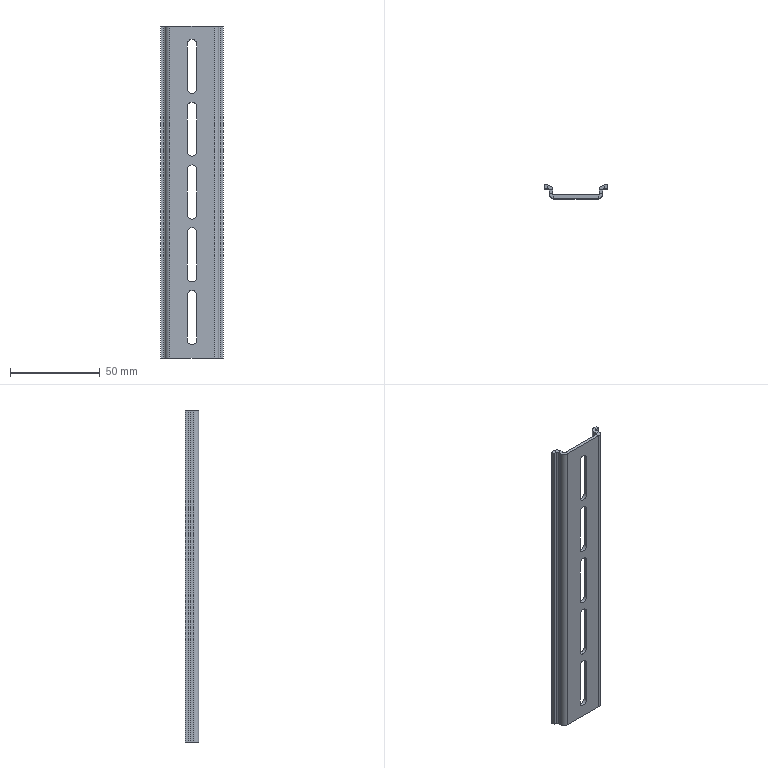Part | STEP file | Guide rail | 1 solid | 63 faces | box 35 x 7.5 x 185 mm | volume 14405 mm3 | plane 40 | cylinder 23 | commonest cylinder face diameters 5.2 x15 1.473 x4 5.473 x4